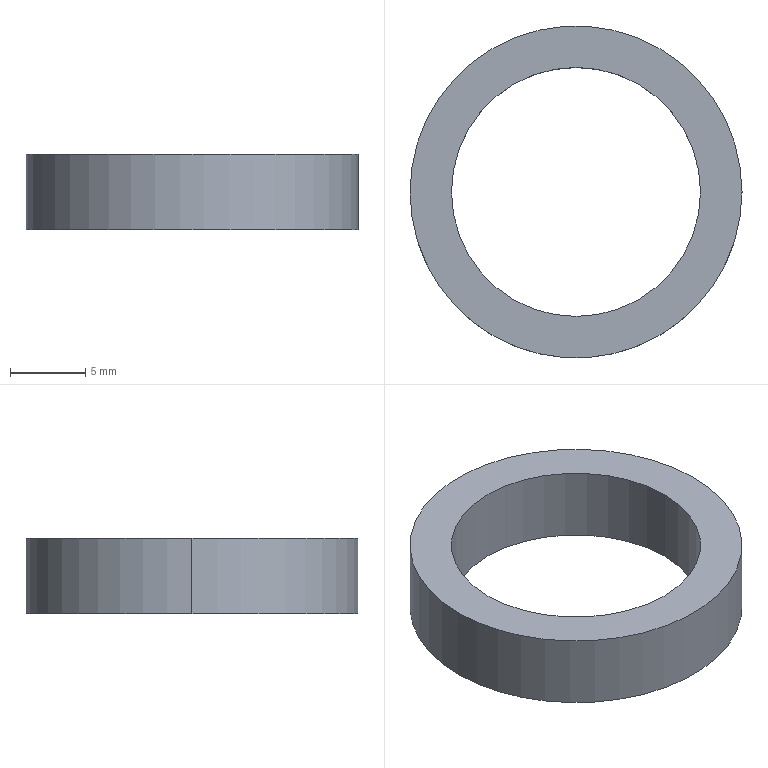Part | SolidWorks | features Extrusion 1 | 1 solid | 6 faces | box 22 x 22 x 5 mm | volume 831.54 mm3 | cylinder 4 | plane 2 | commonest cylinder face diameters 16.5 x2 22 x2
STEP:
#1=CARTESIAN_POINT('',(-8.25,0.,2.5));
#2=VERTEX_POINT('',#1);
#3=CARTESIAN_POINT('',(8.25,0.,2.5));
#4=VERTEX_POINT('',#3);
#5=CARTESIAN_POINT('',(0.,0.,2.5));
#6=DIRECTION('',(0.,0.,1.));
#7=DIRECTION('',(1.,0.,0.));
#8=AXIS2_PLACEMENT_3D('',#5,#6,#7);
#9=CIRCLE('',#8,8.25);
#10=EDGE_CURVE('',#2,#4,#9,.T.);
#11=ORIENTED_EDGE('',*,*,#10,.T.);
#12=CARTESIAN_POINT('',(8.25,0.,-2.5));
#13=VERTEX_POINT('',#12);
#14=CARTESIAN_POINT('',(8.25,0.,2.5));
#15=DIRECTION('',(0.,0.,-1.));
#16=VECTOR('',#15,1000.);
#17=LINE('',#14,#16);
#18=EDGE_CURVE('',#4,#13,#17,.T.);
#19=ORIENTED_EDGE('',*,*,#18,.T.);
#20=CARTESIAN_POINT('',(-8.25,0.,-2.5));
#21=VERTEX_POINT('',#20);
#22=CARTESIAN_POINT('',(0.,0.,-2.5));
#23=DIRECTION('',(0.,0.,1.));
#24=DIRECTION('',(1.,0.,0.));
#25=AXIS2_PLACEMENT_3D('',#22,#23,#24);
#26=CIRCLE('',#25,8.25);
#27=EDGE_CURVE('',#21,#13,#26,.T.);
#28=ORIENTED_EDGE('',*,*,#27,.F.);
#29=CARTESIAN_POINT('',(-8.25,0.,2.5));
#30=DIRECTION('',(0.,0.,-1.));
#31=VECTOR('',#30,1000.);
#32=LINE('',#29,#31);
#33=EDGE_CURVE('',#2,#21,#32,.T.);
#34=ORIENTED_EDGE('',*,*,#33,.F.);
#35=EDGE_LOOP('',(#11,#19,#28,#34));
#36=FACE_OUTER_BOUND('',#35,.T.);
#37=CARTESIAN_POINT('',(0.,0.,2.5));
#38=DIRECTION('',(0.,0.,-1.));
#39=DIRECTION('',(-1.,0.,0.));
#40=AXIS2_PLACEMENT_3D('',#37,#38,#39);
#41=CYLINDRICAL_SURFACE('',#40,8.25);
#42=ADVANCED_FACE('',(#36),#41,.F.);
#43=CARTESIAN_POINT('',(11.,0.,2.5));
#44=VERTEX_POINT('',#43);
#45=CARTESIAN_POINT('',(-11.,0.,2.5));
#46=VERTEX_POINT('',#45);
#47=CARTESIAN_POINT('',(0.,0.,2.5));
#48=DIRECTION('',(0.,0.,1.));
#49=DIRECTION('',(1.,0.,0.));
#50=AXIS2_PLACEMENT_3D('',#47,#48,#49);
#51=CIRCLE('',#50,11.);
#52=EDGE_CURVE('',#44,#46,#51,.T.);
#53=ORIENTED_EDGE('',*,*,#52,.F.);
#54=CARTESIAN_POINT('',(11.,0.,-2.5));
#55=VERTEX_POINT('',#54);
#56=CARTESIAN_POINT('',(11.,0.,2.5));
#57=DIRECTION('',(0.,0.,-1.));
#58=VECTOR('',#57,1000.);
#59=LINE('',#56,#58);
#60=EDGE_CURVE('',#44,#55,#59,.T.);
#61=ORIENTED_EDGE('',*,*,#60,.T.);
#62=CARTESIAN_POINT('',(-11.,0.,-2.5));
#63=VERTEX_POINT('',#62);
#64=CARTESIAN_POINT('',(0.,0.,-2.5));
#65=DIRECTION('',(0.,0.,1.));
#66=DIRECTION('',(1.,0.,0.));
#67=AXIS2_PLACEMENT_3D('',#64,#65,#66);
#68=CIRCLE('',#67,11.);
#69=EDGE_CURVE('',#55,#63,#68,.T.);
#70=ORIENTED_EDGE('',*,*,#69,.T.);
#71=CARTESIAN_POINT('',(-11.,0.,2.5));
#72=DIRECTION('',(0.,0.,-1.));
#73=VECTOR('',#72,1000.);
#74=LINE('',#71,#73);
#75=EDGE_CURVE('',#46,#63,#74,.T.);
#76=ORIENTED_EDGE('',*,*,#75,.F.);
#77=EDGE_LOOP('',(#53,#61,#70,#76));
#78=FACE_OUTER_BOUND('',#77,.T.);
#79=CARTESIAN_POINT('',(0.,0.,2.5));
#80=DIRECTION('',(0.,0.,-1.));
#81=DIRECTION('',(-1.,0.,0.));
#82=AXIS2_PLACEMENT_3D('',#79,#80,#81);
#83=CYLINDRICAL_SURFACE('',#82,11.);
#84=ADVANCED_FACE('',(#78),#83,.T.);
#85=CARTESIAN_POINT('',(0.,0.,2.5));
#86=DIRECTION('',(0.,0.,1.));
#87=DIRECTION('',(1.,0.,0.));
#88=AXIS2_PLACEMENT_3D('',#85,#86,#87);
#89=CIRCLE('',#88,11.);
#90=EDGE_CURVE('',#46,#44,#89,.T.);
#91=ORIENTED_EDGE('',*,*,#90,.T.);
#92=ORIENTED_EDGE('',*,*,#52,.T.);
#93=EDGE_LOOP('',(#91,#92));
#94=FACE_OUTER_BOUND('',#93,.T.);
#95=ORIENTED_EDGE('',*,*,#10,.F.);
#96=CARTESIAN_POINT('',(0.,0.,2.5));
#97=DIRECTION('',(0.,0.,1.));
#98=DIRECTION('',(1.,0.,0.));
#99=AXIS2_PLACEMENT_3D('',#96,#97,#98);
#100=CIRCLE('',#99,8.25);
#101=EDGE_CURVE('',#4,#2,#100,.T.);
#102=ORIENTED_EDGE('',*,*,#101,.F.);
#103=EDGE_LOOP('',(#95,#102));
#104=FACE_BOUND('',#103,.T.);
#105=CARTESIAN_POINT('',(0.,0.,2.5));
#106=DIRECTION('',(0.,0.,1.));
#107=DIRECTION('',(1.,0.,0.));
#108=AXIS2_PLACEMENT_3D('',#105,#106,#107);
#109=PLANE('',#108);
#110=ADVANCED_FACE('',(#94,#104),#109,.T.);
#111=CARTESIAN_POINT('',(0.,0.,-2.5));
#112=DIRECTION('',(0.,0.,1.));
#113=DIRECTION('',(1.,0.,0.));
#114=AXIS2_PLACEMENT_3D('',#111,#112,#113);
#115=CIRCLE('',#114,11.);
#116=EDGE_CURVE('',#63,#55,#115,.T.);
#117=ORIENTED_EDGE('',*,*,#116,.F.);
#118=ORIENTED_EDGE('',*,*,#69,.F.);
#119=EDGE_LOOP('',(#117,#118));
#120=FACE_OUTER_BOUND('',#119,.T.);
#121=ORIENTED_EDGE('',*,*,#27,.T.);
#122=CARTESIAN_POINT('',(0.,0.,-2.5));
#123=DIRECTION('',(0.,0.,1.));
#124=DIRECTION('',(1.,0.,0.));
#125=AXIS2_PLACEMENT_3D('',#122,#123,#124);
#126=CIRCLE('',#125,8.25);
#127=EDGE_CURVE('',#13,#21,#126,.T.);
#128=ORIENTED_EDGE('',*,*,#127,.T.);
#129=EDGE_LOOP('',(#121,#128));
#130=FACE_BOUND('',#129,.T.);
#131=CARTESIAN_POINT('',(0.,0.,-2.5));
#132=DIRECTION('',(0.,0.,1.));
#133=DIRECTION('',(1.,0.,0.));
#134=AXIS2_PLACEMENT_3D('',#131,#132,#133);
#135=PLANE('',#134);
#136=ADVANCED_FACE('',(#120,#130),#135,.F.);
#137=ORIENTED_EDGE('',*,*,#60,.F.);
#138=ORIENTED_EDGE('',*,*,#90,.F.);
#139=ORIENTED_EDGE('',*,*,#75,.T.);
#140=ORIENTED_EDGE('',*,*,#116,.T.);
#141=EDGE_LOOP('',(#137,#138,#139,#140));
#142=FACE_OUTER_BOUND('',#141,.T.);
#143=CARTESIAN_POINT('',(0.,0.,2.5));
#144=DIRECTION('',(0.,0.,-1.));
#145=DIRECTION('',(-1.,0.,0.));
#146=AXIS2_PLACEMENT_3D('',#143,#144,#145);
#147=CYLINDRICAL_SURFACE('',#146,11.);
#148=ADVANCED_FACE('',(#142),#147,.T.);
#149=ORIENTED_EDGE('',*,*,#18,.F.);
#150=ORIENTED_EDGE('',*,*,#101,.T.);
#151=ORIENTED_EDGE('',*,*,#33,.T.);
#152=ORIENTED_EDGE('',*,*,#127,.F.);
#153=EDGE_LOOP('',(#149,#150,#151,#152));
#154=FACE_OUTER_BOUND('',#153,.T.);
#155=CARTESIAN_POINT('',(0.,0.,2.5));
#156=DIRECTION('',(0.,0.,-1.));
#157=DIRECTION('',(-1.,0.,0.));
#158=AXIS2_PLACEMENT_3D('',#155,#156,#157);
#159=CYLINDRICAL_SURFACE('',#158,8.25);
#160=ADVANCED_FACE('',(#154),#159,.F.);
#161=CLOSED_SHELL('',(#42,#84,#110,#136,#148,#160));
#162=MANIFOLD_SOLID_BREP('',#161);
#163=CARTESIAN_POINT('',(0.,0.,0.));
#164=DIRECTION('',(0.,0.,1.));
#165=DIRECTION('',(1.,0.,0.));
#166=AXIS2_PLACEMENT_3D('',#163,#164,#165);
#167=(LENGTH_UNIT()NAMED_UNIT(*)SI_UNIT(.MILLI.,.METRE.));
#168=UNCERTAINTY_MEASURE_WITH_UNIT(LENGTH_MEASURE(0.00001),#167,'','');
#169=(NAMED_UNIT(*)PLANE_ANGLE_UNIT()SI_UNIT($,.RADIAN.));
#170=(NAMED_UNIT(*)SI_UNIT($,.STERADIAN.)SOLID_ANGLE_UNIT());
#171=(GEOMETRIC_REPRESENTATION_CONTEXT(3)GLOBAL_UNCERTAINTY_ASSIGNED_CONTEXT((#168))GLOBAL_UNIT_ASSIGNED_CONTEXT((#167,#169,#170))REPRESENTATION_CONTEXT('',''));
#172=ADVANCED_BREP_SHAPE_REPRESENTATION('',(#162,#166),#171);